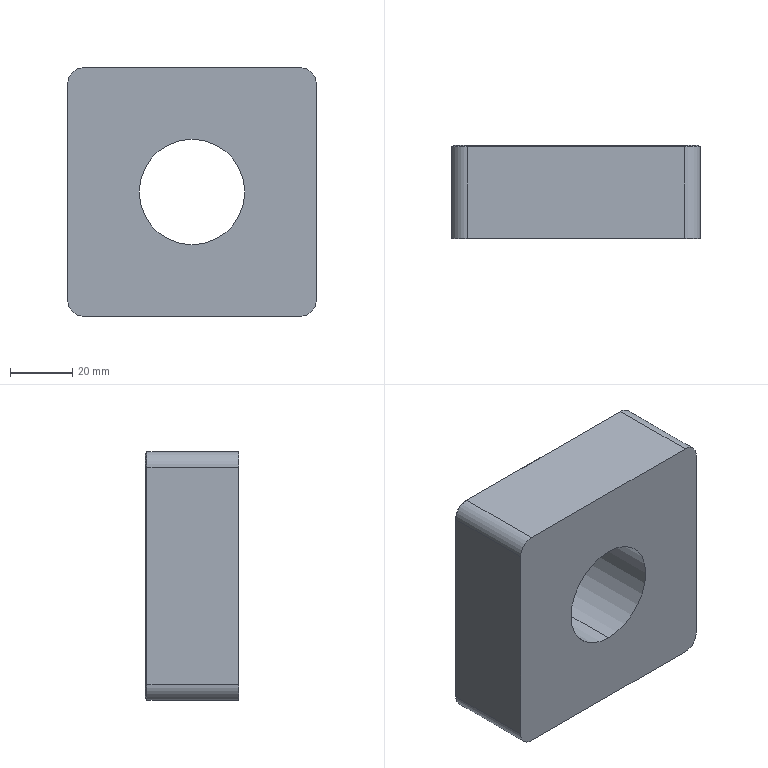Part | SolidWorks | features Chamfer 1, Extrusion 1, Fillet 1, HoleWzd 1 | 1 solid | 20 faces | box 80 x 30 x 80 mm | volume 164080 mm3 | plane 10 | cylinder 6 | cone 4 | commonest cylinder face diameters 10 x4 34 x2
STEP:
#1=CARTESIAN_POINT('',(0.,0.,-17.));
#2=VERTEX_POINT('',#1);
#3=CARTESIAN_POINT('',(0.,0.,17.));
#4=VERTEX_POINT('',#3);
#5=CARTESIAN_POINT('',(0.,0.,0.));
#6=DIRECTION('',(0.,1.,0.));
#7=DIRECTION('',(0.,0.,1.));
#8=AXIS2_PLACEMENT_3D('',#5,#6,#7);
#9=CIRCLE('',#8,17.);
#10=EDGE_CURVE('',#2,#4,#9,.T.);
#11=ORIENTED_EDGE('',*,*,#10,.F.);
#12=CARTESIAN_POINT('',(0.,30.,-17.));
#13=VERTEX_POINT('',#12);
#14=CARTESIAN_POINT('',(0.,30.,-17.));
#15=DIRECTION('',(0.,1.,0.));
#16=VECTOR('',#15,1000.);
#17=LINE('',#14,#16);
#18=EDGE_CURVE('',#2,#13,#17,.T.);
#19=ORIENTED_EDGE('',*,*,#18,.T.);
#20=CARTESIAN_POINT('',(0.,30.,17.));
#21=VERTEX_POINT('',#20);
#22=CARTESIAN_POINT('',(0.,30.,0.));
#23=DIRECTION('',(0.,1.,0.));
#24=DIRECTION('',(0.,0.,1.));
#25=AXIS2_PLACEMENT_3D('',#22,#23,#24);
#26=CIRCLE('',#25,17.);
#27=EDGE_CURVE('',#13,#21,#26,.T.);
#28=ORIENTED_EDGE('',*,*,#27,.T.);
#29=CARTESIAN_POINT('',(0.,30.,17.));
#30=DIRECTION('',(0.,1.,0.));
#31=VECTOR('',#30,1000.);
#32=LINE('',#29,#31);
#33=EDGE_CURVE('',#4,#21,#32,.T.);
#34=ORIENTED_EDGE('',*,*,#33,.F.);
#35=EDGE_LOOP('',(#11,#19,#28,#34));
#36=FACE_OUTER_BOUND('',#35,.T.);
#37=CARTESIAN_POINT('',(0.,30.,0.));
#38=DIRECTION('',(0.,1.,0.));
#39=DIRECTION('',(0.,0.,1.));
#40=AXIS2_PLACEMENT_3D('',#37,#38,#39);
#41=CYLINDRICAL_SURFACE('',#40,17.);
#42=ADVANCED_FACE('',(#36),#41,.F.);
#43=CARTESIAN_POINT('',(-40.,0.,35.));
#44=VERTEX_POINT('',#43);
#45=CARTESIAN_POINT('',(-40.,29.5,35.));
#46=VERTEX_POINT('',#45);
#47=CARTESIAN_POINT('',(-40.,0.,35.));
#48=DIRECTION('',(0.,1.,0.));
#49=VECTOR('',#48,1000.);
#50=LINE('',#47,#49);
#51=EDGE_CURVE('',#44,#46,#50,.T.);
#52=ORIENTED_EDGE('',*,*,#51,.T.);
#53=CARTESIAN_POINT('',(-40.,29.5,-35.));
#54=VERTEX_POINT('',#53);
#55=CARTESIAN_POINT('',(-40.,29.5,-40.));
#56=DIRECTION('',(0.,0.,-1.));
#57=VECTOR('',#56,1000.);
#58=LINE('',#55,#57);
#59=EDGE_CURVE('',#46,#54,#58,.T.);
#60=ORIENTED_EDGE('',*,*,#59,.T.);
#61=CARTESIAN_POINT('',(-40.,0.,-35.));
#62=VERTEX_POINT('',#61);
#63=CARTESIAN_POINT('',(-40.,0.,-35.));
#64=DIRECTION('',(0.,-1.,0.));
#65=VECTOR('',#64,1000.);
#66=LINE('',#63,#65);
#67=EDGE_CURVE('',#54,#62,#66,.T.);
#68=ORIENTED_EDGE('',*,*,#67,.T.);
#69=CARTESIAN_POINT('',(-40.,0.,-40.));
#70=DIRECTION('',(0.,0.,1.));
#71=VECTOR('',#70,1000.);
#72=LINE('',#69,#71);
#73=EDGE_CURVE('',#62,#44,#72,.T.);
#74=ORIENTED_EDGE('',*,*,#73,.T.);
#75=EDGE_LOOP('',(#52,#60,#68,#74));
#76=FACE_OUTER_BOUND('',#75,.T.);
#77=CARTESIAN_POINT('',(-40.,0.,-40.));
#78=DIRECTION('',(-1.,0.,0.));
#79=DIRECTION('',(0.,0.,1.));
#80=AXIS2_PLACEMENT_3D('',#77,#78,#79);
#81=PLANE('',#80);
#82=ADVANCED_FACE('',(#76),#81,.T.);
#83=CARTESIAN_POINT('',(-35.,0.,-40.));
#84=VERTEX_POINT('',#83);
#85=CARTESIAN_POINT('',(-35.,29.5,-40.));
#86=VERTEX_POINT('',#85);
#87=CARTESIAN_POINT('',(-35.,0.,-40.));
#88=DIRECTION('',(0.,1.,0.));
#89=VECTOR('',#88,1000.);
#90=LINE('',#87,#89);
#91=EDGE_CURVE('',#84,#86,#90,.T.);
#92=ORIENTED_EDGE('',*,*,#91,.T.);
#93=CARTESIAN_POINT('',(35.,29.5,-40.));
#94=VERTEX_POINT('',#93);
#95=CARTESIAN_POINT('',(40.,29.5,-40.));
#96=DIRECTION('',(1.,0.,0.));
#97=VECTOR('',#96,1000.);
#98=LINE('',#95,#97);
#99=EDGE_CURVE('',#86,#94,#98,.T.);
#100=ORIENTED_EDGE('',*,*,#99,.T.);
#101=CARTESIAN_POINT('',(35.,0.,-40.));
#102=VERTEX_POINT('',#101);
#103=CARTESIAN_POINT('',(35.,0.,-40.));
#104=DIRECTION('',(0.,-1.,0.));
#105=VECTOR('',#104,1000.);
#106=LINE('',#103,#105);
#107=EDGE_CURVE('',#94,#102,#106,.T.);
#108=ORIENTED_EDGE('',*,*,#107,.T.);
#109=CARTESIAN_POINT('',(40.,0.,-40.));
#110=DIRECTION('',(-1.,0.,0.));
#111=VECTOR('',#110,1000.);
#112=LINE('',#109,#111);
#113=EDGE_CURVE('',#102,#84,#112,.T.);
#114=ORIENTED_EDGE('',*,*,#113,.T.);
#115=EDGE_LOOP('',(#92,#100,#108,#114));
#116=FACE_OUTER_BOUND('',#115,.T.);
#117=CARTESIAN_POINT('',(40.,0.,-40.));
#118=DIRECTION('',(0.,0.,-1.));
#119=DIRECTION('',(-1.,0.,0.));
#120=AXIS2_PLACEMENT_3D('',#117,#118,#119);
#121=PLANE('',#120);
#122=ADVANCED_FACE('',(#116),#121,.T.);
#123=CARTESIAN_POINT('',(40.,0.,-35.));
#124=VERTEX_POINT('',#123);
#125=CARTESIAN_POINT('',(40.,29.5,-35.));
#126=VERTEX_POINT('',#125);
#127=CARTESIAN_POINT('',(40.,0.,-35.));
#128=DIRECTION('',(0.,1.,0.));
#129=VECTOR('',#128,1000.);
#130=LINE('',#127,#129);
#131=EDGE_CURVE('',#124,#126,#130,.T.);
#132=ORIENTED_EDGE('',*,*,#131,.T.);
#133=CARTESIAN_POINT('',(40.,29.5,35.));
#134=VERTEX_POINT('',#133);
#135=CARTESIAN_POINT('',(40.,29.5,40.));
#136=DIRECTION('',(0.,0.,1.));
#137=VECTOR('',#136,1000.);
#138=LINE('',#135,#137);
#139=EDGE_CURVE('',#126,#134,#138,.T.);
#140=ORIENTED_EDGE('',*,*,#139,.T.);
#141=CARTESIAN_POINT('',(40.,0.,35.));
#142=VERTEX_POINT('',#141);
#143=CARTESIAN_POINT('',(40.,0.,35.));
#144=DIRECTION('',(0.,-1.,0.));
#145=VECTOR('',#144,1000.);
#146=LINE('',#143,#145);
#147=EDGE_CURVE('',#134,#142,#146,.T.);
#148=ORIENTED_EDGE('',*,*,#147,.T.);
#149=CARTESIAN_POINT('',(40.,0.,40.));
#150=DIRECTION('',(0.,0.,-1.));
#151=VECTOR('',#150,1000.);
#152=LINE('',#149,#151);
#153=EDGE_CURVE('',#142,#124,#152,.T.);
#154=ORIENTED_EDGE('',*,*,#153,.T.);
#155=EDGE_LOOP('',(#132,#140,#148,#154));
#156=FACE_OUTER_BOUND('',#155,.T.);
#157=CARTESIAN_POINT('',(40.,0.,40.));
#158=DIRECTION('',(1.,0.,0.));
#159=DIRECTION('',(0.,0.,-1.));
#160=AXIS2_PLACEMENT_3D('',#157,#158,#159);
#161=PLANE('',#160);
#162=ADVANCED_FACE('',(#156),#161,.T.);
#163=CARTESIAN_POINT('',(35.,0.,40.));
#164=VERTEX_POINT('',#163);
#165=CARTESIAN_POINT('',(35.,29.5,40.));
#166=VERTEX_POINT('',#165);
#167=CARTESIAN_POINT('',(35.,0.,40.));
#168=DIRECTION('',(0.,1.,0.));
#169=VECTOR('',#168,1000.);
#170=LINE('',#167,#169);
#171=EDGE_CURVE('',#164,#166,#170,.T.);
#172=ORIENTED_EDGE('',*,*,#171,.T.);
#173=CARTESIAN_POINT('',(-35.,29.5,40.));
#174=VERTEX_POINT('',#173);
#175=CARTESIAN_POINT('',(-40.,29.5,40.));
#176=DIRECTION('',(-1.,0.,0.));
#177=VECTOR('',#176,1000.);
#178=LINE('',#175,#177);
#179=EDGE_CURVE('',#166,#174,#178,.T.);
#180=ORIENTED_EDGE('',*,*,#179,.T.);
#181=CARTESIAN_POINT('',(-35.,0.,40.));
#182=VERTEX_POINT('',#181);
#183=CARTESIAN_POINT('',(-35.,0.,40.));
#184=DIRECTION('',(0.,-1.,0.));
#185=VECTOR('',#184,1000.);
#186=LINE('',#183,#185);
#187=EDGE_CURVE('',#174,#182,#186,.T.);
#188=ORIENTED_EDGE('',*,*,#187,.T.);
#189=CARTESIAN_POINT('',(-40.,0.,40.));
#190=DIRECTION('',(1.,0.,0.));
#191=VECTOR('',#190,1000.);
#192=LINE('',#189,#191);
#193=EDGE_CURVE('',#182,#164,#192,.T.);
#194=ORIENTED_EDGE('',*,*,#193,.T.);
#195=EDGE_LOOP('',(#172,#180,#188,#194));
#196=FACE_OUTER_BOUND('',#195,.T.);
#197=CARTESIAN_POINT('',(-40.,0.,40.));
#198=DIRECTION('',(0.,0.,1.));
#199=DIRECTION('',(1.,0.,0.));
#200=AXIS2_PLACEMENT_3D('',#197,#198,#199);
#201=PLANE('',#200);
#202=ADVANCED_FACE('',(#196),#201,.T.);
#203=CARTESIAN_POINT('',(0.,0.,0.));
#204=DIRECTION('',(0.,1.,0.));
#205=DIRECTION('',(0.,0.,1.));
#206=AXIS2_PLACEMENT_3D('',#203,#204,#205);
#207=CIRCLE('',#206,17.);
#208=EDGE_CURVE('',#4,#2,#207,.T.);
#209=ORIENTED_EDGE('',*,*,#208,.T.);
#210=ORIENTED_EDGE('',*,*,#10,.T.);
#211=EDGE_LOOP('',(#209,#210));
#212=FACE_BOUND('',#211,.T.);
#213=ORIENTED_EDGE('',*,*,#153,.F.);
#214=CARTESIAN_POINT('',(35.,0.,35.));
#215=DIRECTION('',(0.,-1.,0.));
#216=DIRECTION('',(0.,0.,1.));
#217=AXIS2_PLACEMENT_3D('',#214,#215,#216);
#218=CIRCLE('',#217,5.);
#219=EDGE_CURVE('',#142,#164,#218,.T.);
#220=ORIENTED_EDGE('',*,*,#219,.T.);
#221=ORIENTED_EDGE('',*,*,#193,.F.);
#222=CARTESIAN_POINT('',(-35.,0.,35.));
#223=DIRECTION('',(0.,-1.,0.));
#224=DIRECTION('',(0.,0.,1.));
#225=AXIS2_PLACEMENT_3D('',#222,#223,#224);
#226=CIRCLE('',#225,5.);
#227=EDGE_CURVE('',#182,#44,#226,.T.);
#228=ORIENTED_EDGE('',*,*,#227,.T.);
#229=ORIENTED_EDGE('',*,*,#73,.F.);
#230=CARTESIAN_POINT('',(-35.,0.,-35.));
#231=DIRECTION('',(0.,-1.,0.));
#232=DIRECTION('',(0.,0.,1.));
#233=AXIS2_PLACEMENT_3D('',#230,#231,#232);
#234=CIRCLE('',#233,5.);
#235=EDGE_CURVE('',#62,#84,#234,.T.);
#236=ORIENTED_EDGE('',*,*,#235,.T.);
#237=ORIENTED_EDGE('',*,*,#113,.F.);
#238=CARTESIAN_POINT('',(35.,0.,-35.));
#239=DIRECTION('',(0.,-1.,0.));
#240=DIRECTION('',(0.,0.,1.));
#241=AXIS2_PLACEMENT_3D('',#238,#239,#240);
#242=CIRCLE('',#241,5.);
#243=EDGE_CURVE('',#102,#124,#242,.T.);
#244=ORIENTED_EDGE('',*,*,#243,.T.);
#245=EDGE_LOOP('',(#213,#220,#221,#228,#229,#236,#237,#244));
#246=FACE_OUTER_BOUND('',#245,.T.);
#247=CARTESIAN_POINT('',(0.,0.,0.));
#248=DIRECTION('',(0.,1.,0.));
#249=DIRECTION('',(0.,0.,1.));
#250=AXIS2_PLACEMENT_3D('',#247,#248,#249);
#251=PLANE('',#250);
#252=ADVANCED_FACE('',(#212,#246),#251,.F.);
#253=CARTESIAN_POINT('',(39.5,30.,-35.));
#254=VERTEX_POINT('',#253);
#255=CARTESIAN_POINT('',(35.,30.,-39.5));
#256=VERTEX_POINT('',#255);
#257=CARTESIAN_POINT('',(35.,30.,-35.));
#258=DIRECTION('',(0.,1.,0.));
#259=DIRECTION('',(0.,0.,1.));
#260=AXIS2_PLACEMENT_3D('',#257,#258,#259);
#261=CIRCLE('',#260,4.5);
#262=EDGE_CURVE('',#254,#256,#261,.T.);
#263=ORIENTED_EDGE('',*,*,#262,.T.);
#264=CARTESIAN_POINT('',(-35.,30.,-39.5));
#265=VERTEX_POINT('',#264);
#266=CARTESIAN_POINT('',(0.,30.,-39.5));
#267=DIRECTION('',(-1.,0.,0.));
#268=VECTOR('',#267,1000.);
#269=LINE('',#266,#268);
#270=EDGE_CURVE('',#256,#265,#269,.T.);
#271=ORIENTED_EDGE('',*,*,#270,.T.);
#272=CARTESIAN_POINT('',(-39.5,30.,-35.));
#273=VERTEX_POINT('',#272);
#274=CARTESIAN_POINT('',(-35.,30.,-35.));
#275=DIRECTION('',(0.,1.,0.));
#276=DIRECTION('',(0.,0.,1.));
#277=AXIS2_PLACEMENT_3D('',#274,#275,#276);
#278=CIRCLE('',#277,4.5);
#279=EDGE_CURVE('',#265,#273,#278,.T.);
#280=ORIENTED_EDGE('',*,*,#279,.T.);
#281=CARTESIAN_POINT('',(-39.5,30.,35.));
#282=VERTEX_POINT('',#281);
#283=CARTESIAN_POINT('',(-39.5,30.,0.));
#284=DIRECTION('',(0.,0.,1.));
#285=VECTOR('',#284,1000.);
#286=LINE('',#283,#285);
#287=EDGE_CURVE('',#273,#282,#286,.T.);
#288=ORIENTED_EDGE('',*,*,#287,.T.);
#289=CARTESIAN_POINT('',(-35.,30.,39.5));
#290=VERTEX_POINT('',#289);
#291=CARTESIAN_POINT('',(-35.,30.,35.));
#292=DIRECTION('',(0.,1.,0.));
#293=DIRECTION('',(0.,0.,1.));
#294=AXIS2_PLACEMENT_3D('',#291,#292,#293);
#295=CIRCLE('',#294,4.5);
#296=EDGE_CURVE('',#282,#290,#295,.T.);
#297=ORIENTED_EDGE('',*,*,#296,.T.);
#298=CARTESIAN_POINT('',(35.,30.,39.5));
#299=VERTEX_POINT('',#298);
#300=CARTESIAN_POINT('',(0.,30.,39.5));
#301=DIRECTION('',(1.,0.,0.));
#302=VECTOR('',#301,1000.);
#303=LINE('',#300,#302);
#304=EDGE_CURVE('',#290,#299,#303,.T.);
#305=ORIENTED_EDGE('',*,*,#304,.T.);
#306=CARTESIAN_POINT('',(39.5,30.,35.));
#307=VERTEX_POINT('',#306);
#308=CARTESIAN_POINT('',(35.,30.,35.));
#309=DIRECTION('',(0.,1.,0.));
#310=DIRECTION('',(0.,0.,1.));
#311=AXIS2_PLACEMENT_3D('',#308,#309,#310);
#312=CIRCLE('',#311,4.5);
#313=EDGE_CURVE('',#299,#307,#312,.T.);
#314=ORIENTED_EDGE('',*,*,#313,.T.);
#315=CARTESIAN_POINT('',(39.5,30.,0.));
#316=DIRECTION('',(0.,0.,-1.));
#317=VECTOR('',#316,1000.);
#318=LINE('',#315,#317);
#319=EDGE_CURVE('',#307,#254,#318,.T.);
#320=ORIENTED_EDGE('',*,*,#319,.T.);
#321=EDGE_LOOP('',(#263,#271,#280,#288,#297,#305,#314,#320));
#322=FACE_OUTER_BOUND('',#321,.T.);
#323=CARTESIAN_POINT('',(0.,30.,0.));
#324=DIRECTION('',(0.,1.,0.));
#325=DIRECTION('',(0.,0.,1.));
#326=AXIS2_PLACEMENT_3D('',#323,#324,#325);
#327=CIRCLE('',#326,17.);
#328=EDGE_CURVE('',#21,#13,#327,.T.);
#329=ORIENTED_EDGE('',*,*,#328,.F.);
#330=ORIENTED_EDGE('',*,*,#27,.F.);
#331=EDGE_LOOP('',(#329,#330));
#332=FACE_BOUND('',#331,.T.);
#333=CARTESIAN_POINT('',(0.,30.,0.));
#334=DIRECTION('',(0.,1.,0.));
#335=DIRECTION('',(0.,0.,1.));
#336=AXIS2_PLACEMENT_3D('',#333,#334,#335);
#337=PLANE('',#336);
#338=ADVANCED_FACE('',(#322,#332),#337,.T.);
#339=ORIENTED_EDGE('',*,*,#18,.F.);
#340=ORIENTED_EDGE('',*,*,#208,.F.);
#341=ORIENTED_EDGE('',*,*,#33,.T.);
#342=ORIENTED_EDGE('',*,*,#328,.T.);
#343=EDGE_LOOP('',(#339,#340,#341,#342));
#344=FACE_OUTER_BOUND('',#343,.T.);
#345=CARTESIAN_POINT('',(0.,30.,0.));
#346=DIRECTION('',(0.,1.,0.));
#347=DIRECTION('',(0.,0.,1.));
#348=AXIS2_PLACEMENT_3D('',#345,#346,#347);
#349=CYLINDRICAL_SURFACE('',#348,17.);
#350=ADVANCED_FACE('',(#344),#349,.F.);
#351=ORIENTED_EDGE('',*,*,#147,.F.);
#352=CARTESIAN_POINT('',(35.,29.5,35.));
#353=DIRECTION('',(0.,-1.,0.));
#354=DIRECTION('',(0.,0.,1.));
#355=AXIS2_PLACEMENT_3D('',#352,#353,#354);
#356=CIRCLE('',#355,5.);
#357=EDGE_CURVE('',#134,#166,#356,.T.);
#358=ORIENTED_EDGE('',*,*,#357,.T.);
#359=ORIENTED_EDGE('',*,*,#171,.F.);
#360=ORIENTED_EDGE('',*,*,#219,.F.);
#361=EDGE_LOOP('',(#351,#358,#359,#360));
#362=FACE_OUTER_BOUND('',#361,.T.);
#363=CARTESIAN_POINT('',(35.,0.,35.));
#364=DIRECTION('',(0.,1.,0.));
#365=DIRECTION('',(0.,0.,1.));
#366=AXIS2_PLACEMENT_3D('',#363,#364,#365);
#367=CYLINDRICAL_SURFACE('',#366,5.);
#368=ADVANCED_FACE('',(#362),#367,.T.);
#369=ORIENTED_EDGE('',*,*,#187,.F.);
#370=CARTESIAN_POINT('',(-35.,29.5,35.));
#371=DIRECTION('',(0.,-1.,0.));
#372=DIRECTION('',(0.,0.,1.));
#373=AXIS2_PLACEMENT_3D('',#370,#371,#372);
#374=CIRCLE('',#373,5.);
#375=EDGE_CURVE('',#174,#46,#374,.T.);
#376=ORIENTED_EDGE('',*,*,#375,.T.);
#377=ORIENTED_EDGE('',*,*,#51,.F.);
#378=ORIENTED_EDGE('',*,*,#227,.F.);
#379=EDGE_LOOP('',(#369,#376,#377,#378));
#380=FACE_OUTER_BOUND('',#379,.T.);
#381=CARTESIAN_POINT('',(-35.,0.,35.));
#382=DIRECTION('',(0.,1.,0.));
#383=DIRECTION('',(0.,0.,1.));
#384=AXIS2_PLACEMENT_3D('',#381,#382,#383);
#385=CYLINDRICAL_SURFACE('',#384,5.);
#386=ADVANCED_FACE('',(#380),#385,.T.);
#387=ORIENTED_EDGE('',*,*,#107,.F.);
#388=CARTESIAN_POINT('',(35.,29.5,-35.));
#389=DIRECTION('',(0.,-1.,0.));
#390=DIRECTION('',(0.,0.,1.));
#391=AXIS2_PLACEMENT_3D('',#388,#389,#390);
#392=CIRCLE('',#391,5.);
#393=EDGE_CURVE('',#94,#126,#392,.T.);
#394=ORIENTED_EDGE('',*,*,#393,.T.);
#395=ORIENTED_EDGE('',*,*,#131,.F.);
#396=ORIENTED_EDGE('',*,*,#243,.F.);
#397=EDGE_LOOP('',(#387,#394,#395,#396));
#398=FACE_OUTER_BOUND('',#397,.T.);
#399=CARTESIAN_POINT('',(35.,0.,-35.));
#400=DIRECTION('',(0.,1.,0.));
#401=DIRECTION('',(0.,0.,1.));
#402=AXIS2_PLACEMENT_3D('',#399,#400,#401);
#403=CYLINDRICAL_SURFACE('',#402,5.);
#404=ADVANCED_FACE('',(#398),#403,.T.);
#405=ORIENTED_EDGE('',*,*,#67,.F.);
#406=CARTESIAN_POINT('',(-35.,29.5,-35.));
#407=DIRECTION('',(0.,-1.,0.));
#408=DIRECTION('',(0.,0.,1.));
#409=AXIS2_PLACEMENT_3D('',#406,#407,#408);
#410=CIRCLE('',#409,5.);
#411=EDGE_CURVE('',#54,#86,#410,.T.);
#412=ORIENTED_EDGE('',*,*,#411,.T.);
#413=ORIENTED_EDGE('',*,*,#91,.F.);
#414=ORIENTED_EDGE('',*,*,#235,.F.);
#415=EDGE_LOOP('',(#405,#412,#413,#414));
#416=FACE_OUTER_BOUND('',#415,.T.);
#417=CARTESIAN_POINT('',(-35.,0.,-35.));
#418=DIRECTION('',(0.,1.,0.));
#419=DIRECTION('',(0.,0.,1.));
#420=AXIS2_PLACEMENT_3D('',#417,#418,#419);
#421=CYLINDRICAL_SURFACE('',#420,5.);
#422=ADVANCED_FACE('',(#416),#421,.T.);
#423=CARTESIAN_POINT('',(-35.,29.5,40.));
#424=DIRECTION('',(0.,0.7071,-0.7071));
#425=VECTOR('',#424,1000.);
#426=LINE('',#423,#425);
#427=EDGE_CURVE('',#174,#290,#426,.T.);
#428=ORIENTED_EDGE('',*,*,#427,.F.);
#429=ORIENTED_EDGE('',*,*,#179,.F.);
#430=CARTESIAN_POINT('',(35.,30.,39.5));
#431=DIRECTION('',(0.,-0.7071,0.7071));
#432=VECTOR('',#431,1000.);
#433=LINE('',#430,#432);
#434=EDGE_CURVE('',#299,#166,#433,.T.);
#435=ORIENTED_EDGE('',*,*,#434,.F.);
#436=ORIENTED_EDGE('',*,*,#304,.F.);
#437=EDGE_LOOP('',(#428,#429,#435,#436));
#438=FACE_OUTER_BOUND('',#437,.T.);
#439=CARTESIAN_POINT('',(0.,30.,39.5));
#440=DIRECTION('',(0.,-0.7071,-0.7071));
#441=DIRECTION('',(1.,0.,0.));
#442=AXIS2_PLACEMENT_3D('',#439,#440,#441);
#443=PLANE('',#442);
#444=ADVANCED_FACE('',(#438),#443,.F.);
#445=ORIENTED_EDGE('',*,*,#434,.T.);
#446=ORIENTED_EDGE('',*,*,#357,.F.);
#447=CARTESIAN_POINT('',(39.5,30.,35.));
#448=DIRECTION('',(0.7071,-0.7071,0.));
#449=VECTOR('',#448,1000.);
#450=LINE('',#447,#449);
#451=EDGE_CURVE('',#307,#134,#450,.T.);
#452=ORIENTED_EDGE('',*,*,#451,.F.);
#453=ORIENTED_EDGE('',*,*,#313,.F.);
#454=EDGE_LOOP('',(#445,#446,#452,#453));
#455=FACE_OUTER_BOUND('',#454,.T.);
#456=CARTESIAN_POINT('',(35.,30.,35.));
#457=DIRECTION('',(0.,-1.,0.));
#458=DIRECTION('',(0.,0.,-1.));
#459=AXIS2_PLACEMENT_3D('',#456,#457,#458);
#460=CONICAL_SURFACE('',#459,4.5,0.7854);
#461=ADVANCED_FACE('',(#455),#460,.T.);
#462=ORIENTED_EDGE('',*,*,#427,.T.);
#463=ORIENTED_EDGE('',*,*,#296,.F.);
#464=CARTESIAN_POINT('',(-40.,29.5,35.));
#465=DIRECTION('',(0.7071,0.7071,0.));
#466=VECTOR('',#465,1000.);
#467=LINE('',#464,#466);
#468=EDGE_CURVE('',#46,#282,#467,.T.);
#469=ORIENTED_EDGE('',*,*,#468,.F.);
#470=ORIENTED_EDGE('',*,*,#375,.F.);
#471=EDGE_LOOP('',(#462,#463,#469,#470));
#472=FACE_OUTER_BOUND('',#471,.T.);
#473=CARTESIAN_POINT('',(-35.,30.,35.));
#474=DIRECTION('',(0.,-1.,0.));
#475=DIRECTION('',(0.,0.,-1.));
#476=AXIS2_PLACEMENT_3D('',#473,#474,#475);
#477=CONICAL_SURFACE('',#476,4.5,0.7854);
#478=ADVANCED_FACE('',(#472),#477,.T.);
#479=ORIENTED_EDGE('',*,*,#451,.T.);
#480=ORIENTED_EDGE('',*,*,#139,.F.);
#481=CARTESIAN_POINT('',(39.5,30.,-35.));
#482=DIRECTION('',(0.7071,-0.7071,0.));
#483=VECTOR('',#482,1000.);
#484=LINE('',#481,#483);
#485=EDGE_CURVE('',#254,#126,#484,.T.);
#486=ORIENTED_EDGE('',*,*,#485,.F.);
#487=ORIENTED_EDGE('',*,*,#319,.F.);
#488=EDGE_LOOP('',(#479,#480,#486,#487));
#489=FACE_OUTER_BOUND('',#488,.T.);
#490=CARTESIAN_POINT('',(39.5,30.,0.));
#491=DIRECTION('',(-0.7071,-0.7071,0.));
#492=DIRECTION('',(0.,0.,-1.));
#493=AXIS2_PLACEMENT_3D('',#490,#491,#492);
#494=PLANE('',#493);
#495=ADVANCED_FACE('',(#489),#494,.F.);
#496=ORIENTED_EDGE('',*,*,#468,.T.);
#497=ORIENTED_EDGE('',*,*,#287,.F.);
#498=CARTESIAN_POINT('',(-40.,29.5,-35.));
#499=DIRECTION('',(0.7071,0.7071,0.));
#500=VECTOR('',#499,1000.);
#501=LINE('',#498,#500);
#502=EDGE_CURVE('',#54,#273,#501,.T.);
#503=ORIENTED_EDGE('',*,*,#502,.F.);
#504=ORIENTED_EDGE('',*,*,#59,.F.);
#505=EDGE_LOOP('',(#496,#497,#503,#504));
#506=FACE_OUTER_BOUND('',#505,.T.);
#507=CARTESIAN_POINT('',(-39.5,30.,0.));
#508=DIRECTION('',(0.7071,-0.7071,0.));
#509=DIRECTION('',(0.,0.,1.));
#510=AXIS2_PLACEMENT_3D('',#507,#508,#509);
#511=PLANE('',#510);
#512=ADVANCED_FACE('',(#506),#511,.F.);
#513=ORIENTED_EDGE('',*,*,#485,.T.);
#514=ORIENTED_EDGE('',*,*,#393,.F.);
#515=CARTESIAN_POINT('',(35.,30.,-39.5));
#516=DIRECTION('',(0.,-0.7071,-0.7071));
#517=VECTOR('',#516,1000.);
#518=LINE('',#515,#517);
#519=EDGE_CURVE('',#256,#94,#518,.T.);
#520=ORIENTED_EDGE('',*,*,#519,.F.);
#521=ORIENTED_EDGE('',*,*,#262,.F.);
#522=EDGE_LOOP('',(#513,#514,#520,#521));
#523=FACE_OUTER_BOUND('',#522,.T.);
#524=CARTESIAN_POINT('',(35.,30.,-35.));
#525=DIRECTION('',(0.,-1.,0.));
#526=DIRECTION('',(0.,0.,-1.));
#527=AXIS2_PLACEMENT_3D('',#524,#525,#526);
#528=CONICAL_SURFACE('',#527,4.5,0.7854);
#529=ADVANCED_FACE('',(#523),#528,.T.);
#530=ORIENTED_EDGE('',*,*,#502,.T.);
#531=ORIENTED_EDGE('',*,*,#279,.F.);
#532=CARTESIAN_POINT('',(-35.,29.5,-40.));
#533=DIRECTION('',(0.,0.7071,0.7071));
#534=VECTOR('',#533,1000.);
#535=LINE('',#532,#534);
#536=EDGE_CURVE('',#86,#265,#535,.T.);
#537=ORIENTED_EDGE('',*,*,#536,.F.);
#538=ORIENTED_EDGE('',*,*,#411,.F.);
#539=EDGE_LOOP('',(#530,#531,#537,#538));
#540=FACE_OUTER_BOUND('',#539,.T.);
#541=CARTESIAN_POINT('',(-35.,30.,-35.));
#542=DIRECTION('',(0.,-1.,0.));
#543=DIRECTION('',(0.,0.,-1.));
#544=AXIS2_PLACEMENT_3D('',#541,#542,#543);
#545=CONICAL_SURFACE('',#544,4.5,0.7854);
#546=ADVANCED_FACE('',(#540),#545,.T.);
#547=ORIENTED_EDGE('',*,*,#519,.T.);
#548=ORIENTED_EDGE('',*,*,#99,.F.);
#549=ORIENTED_EDGE('',*,*,#536,.T.);
#550=ORIENTED_EDGE('',*,*,#270,.F.);
#551=EDGE_LOOP('',(#547,#548,#549,#550));
#552=FACE_OUTER_BOUND('',#551,.T.);
#553=CARTESIAN_POINT('',(0.,30.,-39.5));
#554=DIRECTION('',(0.,-0.7071,0.7071));
#555=DIRECTION('',(-1.,0.,0.));
#556=AXIS2_PLACEMENT_3D('',#553,#554,#555);
#557=PLANE('',#556);
#558=ADVANCED_FACE('',(#552),#557,.F.);
#559=CLOSED_SHELL('',(#42,#82,#122,#162,#202,#252,#338,#350,#368,#386,#404,#422,#444,#461,#478,#495,#512,#529,#546,#558));
#560=MANIFOLD_SOLID_BREP('',#559);
#561=CARTESIAN_POINT('',(0.,0.,0.));
#562=DIRECTION('',(0.,0.,1.));
#563=DIRECTION('',(1.,0.,0.));
#564=AXIS2_PLACEMENT_3D('',#561,#562,#563);
#565=(LENGTH_UNIT()NAMED_UNIT(*)SI_UNIT(.MILLI.,.METRE.));
#566=UNCERTAINTY_MEASURE_WITH_UNIT(LENGTH_MEASURE(0.00001),#565,'','');
#567=(NAMED_UNIT(*)PLANE_ANGLE_UNIT()SI_UNIT($,.RADIAN.));
#568=(NAMED_UNIT(*)SI_UNIT($,.STERADIAN.)SOLID_ANGLE_UNIT());
#569=(GEOMETRIC_REPRESENTATION_CONTEXT(3)GLOBAL_UNCERTAINTY_ASSIGNED_CONTEXT((#566))GLOBAL_UNIT_ASSIGNED_CONTEXT((#565,#567,#568))REPRESENTATION_CONTEXT('',''));
#570=ADVANCED_BREP_SHAPE_REPRESENTATION('',(#560,#564),#569);